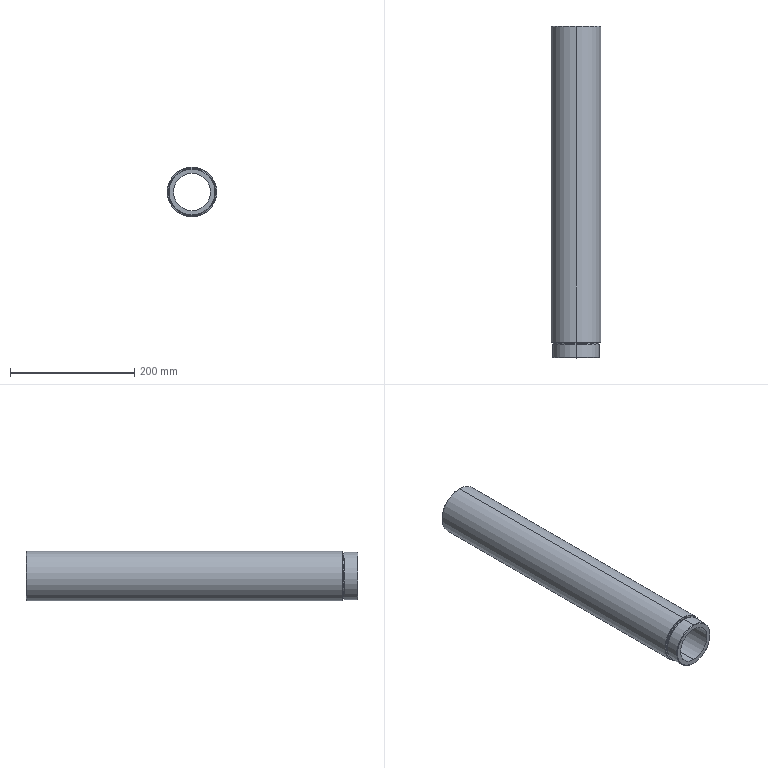Part | SolidWorks | features ICE 8, Chamfer 7, HoleWzd 2, Extrusion 1, Fillet 1 | 1 solid | 33 faces | box 80 x 534.5 x 80 mm | volume 1149532 mm3 | cone 12 | cylinder 12 | plane 5 | torus 4 | commonest cylinder face diameters 60 x2 61 x2 70 x2 73.5 x2 76 x2 80 x2
STEP:
#1=CARTESIAN_POINT('',(0.,529.5,-30.5));
#2=VERTEX_POINT('',#1);
#3=CARTESIAN_POINT('',(0.,529.5,30.5));
#4=VERTEX_POINT('',#3);
#5=CARTESIAN_POINT('',(0.,529.5,0.));
#6=DIRECTION('',(0.,1.,0.));
#7=DIRECTION('',(0.,0.,1.));
#8=AXIS2_PLACEMENT_3D('',#5,#6,#7);
#9=CIRCLE('',#8,30.5);
#10=EDGE_CURVE('',#2,#4,#9,.T.);
#11=ORIENTED_EDGE('',*,*,#10,.F.);
#12=CARTESIAN_POINT('',(0.,530.5,-31.5));
#13=VERTEX_POINT('',#12);
#14=CARTESIAN_POINT('',(0.,529.5,-30.5));
#15=DIRECTION('',(0.,0.7071,-0.7071));
#16=VECTOR('',#15,1000.);
#17=LINE('',#14,#16);
#18=EDGE_CURVE('',#2,#13,#17,.T.);
#19=ORIENTED_EDGE('',*,*,#18,.T.);
#20=CARTESIAN_POINT('',(0.,530.5,31.5));
#21=VERTEX_POINT('',#20);
#22=CARTESIAN_POINT('',(0.,530.5,0.));
#23=DIRECTION('',(0.,-1.,0.));
#24=DIRECTION('',(0.,0.,1.));
#25=AXIS2_PLACEMENT_3D('',#22,#23,#24);
#26=CIRCLE('',#25,31.5);
#27=EDGE_CURVE('',#21,#13,#26,.T.);
#28=ORIENTED_EDGE('',*,*,#27,.F.);
#29=CARTESIAN_POINT('',(0.,529.5,30.5));
#30=DIRECTION('',(0.,0.7071,0.7071));
#31=VECTOR('',#30,1000.);
#32=LINE('',#29,#31);
#33=EDGE_CURVE('',#4,#21,#32,.T.);
#34=ORIENTED_EDGE('',*,*,#33,.F.);
#35=EDGE_LOOP('',(#11,#19,#28,#34));
#36=FACE_OUTER_BOUND('',#35,.T.);
#37=CARTESIAN_POINT('',(0.,529.5,0.));
#38=DIRECTION('',(0.,1.,0.));
#39=DIRECTION('',(0.,0.,1.));
#40=AXIS2_PLACEMENT_3D('',#37,#38,#39);
#41=CONICAL_SURFACE('',#40,30.5,0.7854);
#42=ADVANCED_FACE('',(#36),#41,.F.);
#43=CARTESIAN_POINT('',(0.,475.5,-30.5));
#44=VERTEX_POINT('',#43);
#45=CARTESIAN_POINT('',(0.,475.5,30.5));
#46=VERTEX_POINT('',#45);
#47=CARTESIAN_POINT('',(0.,475.5,0.));
#48=DIRECTION('',(0.,1.,0.));
#49=DIRECTION('',(0.,0.,1.));
#50=AXIS2_PLACEMENT_3D('',#47,#48,#49);
#51=CIRCLE('',#50,30.5);
#52=EDGE_CURVE('',#44,#46,#51,.T.);
#53=ORIENTED_EDGE('',*,*,#52,.F.);
#54=CARTESIAN_POINT('',(0.,530.5,-30.5));
#55=DIRECTION('',(0.,1.,0.));
#56=VECTOR('',#55,1000.);
#57=LINE('',#54,#56);
#58=EDGE_CURVE('',#44,#2,#57,.T.);
#59=ORIENTED_EDGE('',*,*,#58,.T.);
#60=ORIENTED_EDGE('',*,*,#10,.T.);
#61=CARTESIAN_POINT('',(0.,530.5,30.5));
#62=DIRECTION('',(0.,1.,0.));
#63=VECTOR('',#62,1000.);
#64=LINE('',#61,#63);
#65=EDGE_CURVE('',#46,#4,#64,.T.);
#66=ORIENTED_EDGE('',*,*,#65,.F.);
#67=EDGE_LOOP('',(#53,#59,#60,#66));
#68=FACE_OUTER_BOUND('',#67,.T.);
#69=CARTESIAN_POINT('',(0.,530.5,0.));
#70=DIRECTION('',(0.,1.,0.));
#71=DIRECTION('',(0.,0.,1.));
#72=AXIS2_PLACEMENT_3D('',#69,#70,#71);
#73=CYLINDRICAL_SURFACE('',#72,30.5);
#74=ADVANCED_FACE('',(#68),#73,.F.);
#75=CARTESIAN_POINT('',(0.,475.2,30.));
#76=VERTEX_POINT('',#75);
#77=CARTESIAN_POINT('',(0.,475.2,-30.));
#78=VERTEX_POINT('',#77);
#79=CARTESIAN_POINT('',(0.,475.2,0.));
#80=DIRECTION('',(0.,-1.,0.));
#81=DIRECTION('',(0.,0.,1.));
#82=AXIS2_PLACEMENT_3D('',#79,#80,#81);
#83=CIRCLE('',#82,30.);
#84=EDGE_CURVE('',#76,#78,#83,.T.);
#85=ORIENTED_EDGE('',*,*,#84,.T.);
#86=CARTESIAN_POINT('',(0.,475.5,-30.5));
#87=DIRECTION('',(0.,0.515,-0.8572));
#88=VECTOR('',#87,1000.);
#89=LINE('',#86,#88);
#90=EDGE_CURVE('',#78,#44,#89,.T.);
#91=ORIENTED_EDGE('',*,*,#90,.T.);
#92=ORIENTED_EDGE('',*,*,#52,.T.);
#93=CARTESIAN_POINT('',(0.,475.5,30.5));
#94=DIRECTION('',(0.,0.515,0.8572));
#95=VECTOR('',#94,1000.);
#96=LINE('',#93,#95);
#97=EDGE_CURVE('',#76,#46,#96,.T.);
#98=ORIENTED_EDGE('',*,*,#97,.F.);
#99=EDGE_LOOP('',(#85,#91,#92,#98));
#100=FACE_OUTER_BOUND('',#99,.T.);
#101=CARTESIAN_POINT('',(0.,475.5,0.));
#102=DIRECTION('',(0.,1.,0.));
#103=DIRECTION('',(0.,0.,1.));
#104=AXIS2_PLACEMENT_3D('',#101,#102,#103);
#105=CONICAL_SURFACE('',#104,30.5,1.03);
#106=ADVANCED_FACE('',(#100),#105,.F.);
#107=CARTESIAN_POINT('',(0.,27.5,36.75));
#108=VERTEX_POINT('',#107);
#109=CARTESIAN_POINT('',(0.,27.5,-36.75));
#110=VERTEX_POINT('',#109);
#111=CARTESIAN_POINT('',(0.,27.5,0.));
#112=DIRECTION('',(0.,-1.,0.));
#113=DIRECTION('',(0.,0.,-1.));
#114=AXIS2_PLACEMENT_3D('',#111,#112,#113);
#115=CIRCLE('',#114,36.75);
#116=EDGE_CURVE('',#108,#110,#115,.T.);
#117=ORIENTED_EDGE('',*,*,#116,.F.);
#118=CARTESIAN_POINT('',(0.,28.,37.25));
#119=VERTEX_POINT('',#118);
#120=CARTESIAN_POINT('',(0.,27.5,37.25));
#121=DIRECTION('',(1.,0.,0.));
#122=DIRECTION('',(0.,0.,-1.));
#123=AXIS2_PLACEMENT_3D('',#120,#121,#122);
#124=CIRCLE('',#123,0.5);
#125=EDGE_CURVE('',#108,#119,#124,.T.);
#126=ORIENTED_EDGE('',*,*,#125,.T.);
#127=CARTESIAN_POINT('',(0.,28.,-37.25));
#128=VERTEX_POINT('',#127);
#129=CARTESIAN_POINT('',(0.,28.,0.));
#130=DIRECTION('',(0.,1.,0.));
#131=DIRECTION('',(0.,0.,-1.));
#132=AXIS2_PLACEMENT_3D('',#129,#130,#131);
#133=CIRCLE('',#132,37.25);
#134=EDGE_CURVE('',#128,#119,#133,.T.);
#135=ORIENTED_EDGE('',*,*,#134,.F.);
#136=CARTESIAN_POINT('',(0.,27.5,-37.25));
#137=DIRECTION('',(-1.,0.,0.));
#138=DIRECTION('',(0.,0.,1.));
#139=AXIS2_PLACEMENT_3D('',#136,#137,#138);
#140=CIRCLE('',#139,0.5);
#141=EDGE_CURVE('',#110,#128,#140,.T.);
#142=ORIENTED_EDGE('',*,*,#141,.F.);
#143=EDGE_LOOP('',(#117,#126,#135,#142));
#144=FACE_OUTER_BOUND('',#143,.T.);
#145=CARTESIAN_POINT('',(0.,27.5,0.));
#146=DIRECTION('',(0.,-1.,0.));
#147=DIRECTION('',(0.,0.,-1.));
#148=AXIS2_PLACEMENT_3D('',#145,#146,#147);
#149=TOROIDAL_SURFACE('',#148,37.25,0.5);
#150=ADVANCED_FACE('',(#144),#149,.F.);
#151=CARTESIAN_POINT('',(0.,25.,37.25));
#152=VERTEX_POINT('',#151);
#153=CARTESIAN_POINT('',(0.,25.,-37.25));
#154=VERTEX_POINT('',#153);
#155=CARTESIAN_POINT('',(0.,25.,0.));
#156=DIRECTION('',(0.,-1.,0.));
#157=DIRECTION('',(0.,0.,-1.));
#158=AXIS2_PLACEMENT_3D('',#155,#156,#157);
#159=CIRCLE('',#158,37.25);
#160=EDGE_CURVE('',#152,#154,#159,.T.);
#161=ORIENTED_EDGE('',*,*,#160,.F.);
#162=CARTESIAN_POINT('',(0.,25.5,36.75));
#163=VERTEX_POINT('',#162);
#164=CARTESIAN_POINT('',(0.,25.5,37.25));
#165=DIRECTION('',(1.,0.,0.));
#166=DIRECTION('',(0.,0.,-1.));
#167=AXIS2_PLACEMENT_3D('',#164,#165,#166);
#168=CIRCLE('',#167,0.5);
#169=EDGE_CURVE('',#152,#163,#168,.T.);
#170=ORIENTED_EDGE('',*,*,#169,.T.);
#171=CARTESIAN_POINT('',(0.,25.5,-36.75));
#172=VERTEX_POINT('',#171);
#173=CARTESIAN_POINT('',(0.,25.5,0.));
#174=DIRECTION('',(0.,1.,0.));
#175=DIRECTION('',(0.,0.,-1.));
#176=AXIS2_PLACEMENT_3D('',#173,#174,#175);
#177=CIRCLE('',#176,36.75);
#178=EDGE_CURVE('',#172,#163,#177,.T.);
#179=ORIENTED_EDGE('',*,*,#178,.F.);
#180=CARTESIAN_POINT('',(0.,25.5,-37.25));
#181=DIRECTION('',(-1.,0.,0.));
#182=DIRECTION('',(0.,0.,1.));
#183=AXIS2_PLACEMENT_3D('',#180,#181,#182);
#184=CIRCLE('',#183,0.5);
#185=EDGE_CURVE('',#154,#172,#184,.T.);
#186=ORIENTED_EDGE('',*,*,#185,.F.);
#187=EDGE_LOOP('',(#161,#170,#179,#186));
#188=FACE_OUTER_BOUND('',#187,.T.);
#189=CARTESIAN_POINT('',(0.,25.5,0.));
#190=DIRECTION('',(0.,-1.,0.));
#191=DIRECTION('',(0.,0.,-1.));
#192=AXIS2_PLACEMENT_3D('',#189,#190,#191);
#193=TOROIDAL_SURFACE('',#192,37.25,0.5);
#194=ADVANCED_FACE('',(#188),#193,.F.);
#195=CARTESIAN_POINT('',(0.,28.,-39.5));
#196=VERTEX_POINT('',#195);
#197=CARTESIAN_POINT('',(0.,28.,39.5));
#198=VERTEX_POINT('',#197);
#199=CARTESIAN_POINT('',(0.,28.,0.));
#200=DIRECTION('',(0.,-1.,0.));
#201=DIRECTION('',(0.,0.,-1.));
#202=AXIS2_PLACEMENT_3D('',#199,#200,#201);
#203=CIRCLE('',#202,39.5);
#204=EDGE_CURVE('',#196,#198,#203,.T.);
#205=ORIENTED_EDGE('',*,*,#204,.F.);
#206=CARTESIAN_POINT('',(0.,28.5,-40.));
#207=VERTEX_POINT('',#206);
#208=CARTESIAN_POINT('',(0.,28.,-39.5));
#209=DIRECTION('',(0.,0.7071,-0.7071));
#210=VECTOR('',#209,1000.);
#211=LINE('',#208,#210);
#212=EDGE_CURVE('',#196,#207,#211,.T.);
#213=ORIENTED_EDGE('',*,*,#212,.T.);
#214=CARTESIAN_POINT('',(0.,28.5,40.));
#215=VERTEX_POINT('',#214);
#216=CARTESIAN_POINT('',(0.,28.5,0.));
#217=DIRECTION('',(0.,1.,0.));
#218=DIRECTION('',(0.,0.,-1.));
#219=AXIS2_PLACEMENT_3D('',#216,#217,#218);
#220=CIRCLE('',#219,40.);
#221=EDGE_CURVE('',#215,#207,#220,.T.);
#222=ORIENTED_EDGE('',*,*,#221,.F.);
#223=CARTESIAN_POINT('',(0.,28.,39.5));
#224=DIRECTION('',(0.,0.7071,0.7071));
#225=VECTOR('',#224,1000.);
#226=LINE('',#223,#225);
#227=EDGE_CURVE('',#198,#215,#226,.T.);
#228=ORIENTED_EDGE('',*,*,#227,.F.);
#229=EDGE_LOOP('',(#205,#213,#222,#228));
#230=FACE_OUTER_BOUND('',#229,.T.);
#231=CARTESIAN_POINT('',(0.,28.,0.));
#232=DIRECTION('',(0.,1.,0.));
#233=DIRECTION('',(0.,0.,1.));
#234=AXIS2_PLACEMENT_3D('',#231,#232,#233);
#235=CONICAL_SURFACE('',#234,39.5,0.7854);
#236=ADVANCED_FACE('',(#230),#235,.T.);
#237=CARTESIAN_POINT('',(0.,3.,-37.));
#238=VERTEX_POINT('',#237);
#239=CARTESIAN_POINT('',(0.,3.,37.));
#240=VERTEX_POINT('',#239);
#241=CARTESIAN_POINT('',(0.,3.,0.));
#242=DIRECTION('',(0.,-1.,0.));
#243=DIRECTION('',(0.,0.,-1.));
#244=AXIS2_PLACEMENT_3D('',#241,#242,#243);
#245=CIRCLE('',#244,37.);
#246=EDGE_CURVE('',#238,#240,#245,.T.);
#247=ORIENTED_EDGE('',*,*,#246,.F.);
#248=CARTESIAN_POINT('',(0.,4.,-38.));
#249=VERTEX_POINT('',#248);
#250=CARTESIAN_POINT('',(0.,4.,-38.));
#251=DIRECTION('',(0.,0.7071,-0.7071));
#252=VECTOR('',#251,1000.);
#253=LINE('',#250,#252);
#254=EDGE_CURVE('',#238,#249,#253,.T.);
#255=ORIENTED_EDGE('',*,*,#254,.T.);
#256=CARTESIAN_POINT('',(0.,4.,38.));
#257=VERTEX_POINT('',#256);
#258=CARTESIAN_POINT('',(0.,4.,0.));
#259=DIRECTION('',(0.,1.,0.));
#260=DIRECTION('',(0.,0.,-1.));
#261=AXIS2_PLACEMENT_3D('',#258,#259,#260);
#262=CIRCLE('',#261,38.);
#263=EDGE_CURVE('',#257,#249,#262,.T.);
#264=ORIENTED_EDGE('',*,*,#263,.F.);
#265=CARTESIAN_POINT('',(0.,4.,38.));
#266=DIRECTION('',(0.,0.7071,0.7071));
#267=VECTOR('',#266,1000.);
#268=LINE('',#265,#267);
#269=EDGE_CURVE('',#240,#257,#268,.T.);
#270=ORIENTED_EDGE('',*,*,#269,.F.);
#271=EDGE_LOOP('',(#247,#255,#264,#270));
#272=FACE_OUTER_BOUND('',#271,.T.);
#273=CARTESIAN_POINT('',(0.,4.,0.));
#274=DIRECTION('',(0.,1.,0.));
#275=DIRECTION('',(0.,0.,1.));
#276=AXIS2_PLACEMENT_3D('',#273,#274,#275);
#277=CONICAL_SURFACE('',#276,38.,0.7854);
#278=ADVANCED_FACE('',(#272),#277,.T.);
#279=CARTESIAN_POINT('',(0.,537.,-35.));
#280=VERTEX_POINT('',#279);
#281=CARTESIAN_POINT('',(0.,537.,35.));
#282=VERTEX_POINT('',#281);
#283=CARTESIAN_POINT('',(0.,537.,0.));
#284=DIRECTION('',(0.,1.,0.));
#285=DIRECTION('',(0.,0.,1.));
#286=AXIS2_PLACEMENT_3D('',#283,#284,#285);
#287=CIRCLE('',#286,35.);
#288=EDGE_CURVE('',#280,#282,#287,.T.);
#289=ORIENTED_EDGE('',*,*,#288,.F.);
#290=CARTESIAN_POINT('',(0.,537.5,-35.5));
#291=VERTEX_POINT('',#290);
#292=CARTESIAN_POINT('',(0.,537.,-35.));
#293=DIRECTION('',(0.,0.7071,-0.7071));
#294=VECTOR('',#293,1000.);
#295=LINE('',#292,#294);
#296=EDGE_CURVE('',#280,#291,#295,.T.);
#297=ORIENTED_EDGE('',*,*,#296,.T.);
#298=CARTESIAN_POINT('',(0.,537.5,35.5));
#299=VERTEX_POINT('',#298);
#300=CARTESIAN_POINT('',(0.,537.5,0.));
#301=DIRECTION('',(0.,-1.,0.));
#302=DIRECTION('',(0.,0.,1.));
#303=AXIS2_PLACEMENT_3D('',#300,#301,#302);
#304=CIRCLE('',#303,35.5);
#305=EDGE_CURVE('',#299,#291,#304,.T.);
#306=ORIENTED_EDGE('',*,*,#305,.F.);
#307=CARTESIAN_POINT('',(0.,537.,35.));
#308=DIRECTION('',(0.,0.7071,0.7071));
#309=VECTOR('',#308,1000.);
#310=LINE('',#307,#309);
#311=EDGE_CURVE('',#282,#299,#310,.T.);
#312=ORIENTED_EDGE('',*,*,#311,.F.);
#313=EDGE_LOOP('',(#289,#297,#306,#312));
#314=FACE_OUTER_BOUND('',#313,.T.);
#315=CARTESIAN_POINT('',(0.,537.,0.));
#316=DIRECTION('',(0.,1.,0.));
#317=DIRECTION('',(0.,0.,1.));
#318=AXIS2_PLACEMENT_3D('',#315,#316,#317);
#319=CONICAL_SURFACE('',#318,35.,0.7854);
#320=ADVANCED_FACE('',(#314),#319,.F.);
#321=CARTESIAN_POINT('',(0.,530.5,-35.));
#322=VERTEX_POINT('',#321);
#323=CARTESIAN_POINT('',(0.,530.5,35.));
#324=VERTEX_POINT('',#323);
#325=CARTESIAN_POINT('',(0.,530.5,0.));
#326=DIRECTION('',(0.,1.,0.));
#327=DIRECTION('',(0.,0.,1.));
#328=AXIS2_PLACEMENT_3D('',#325,#326,#327);
#329=CIRCLE('',#328,35.);
#330=EDGE_CURVE('',#322,#324,#329,.T.);
#331=ORIENTED_EDGE('',*,*,#330,.F.);
#332=CARTESIAN_POINT('',(0.,530.5,-35.));
#333=DIRECTION('',(0.,1.,0.));
#334=VECTOR('',#333,1000.);
#335=LINE('',#332,#334);
#336=EDGE_CURVE('',#322,#280,#335,.T.);
#337=ORIENTED_EDGE('',*,*,#336,.T.);
#338=ORIENTED_EDGE('',*,*,#288,.T.);
#339=CARTESIAN_POINT('',(0.,530.5,35.));
#340=DIRECTION('',(0.,1.,0.));
#341=VECTOR('',#340,1000.);
#342=LINE('',#339,#341);
#343=EDGE_CURVE('',#324,#282,#342,.T.);
#344=ORIENTED_EDGE('',*,*,#343,.F.);
#345=EDGE_LOOP('',(#331,#337,#338,#344));
#346=FACE_OUTER_BOUND('',#345,.T.);
#347=CARTESIAN_POINT('',(0.,530.5,0.));
#348=DIRECTION('',(0.,1.,0.));
#349=DIRECTION('',(0.,0.,1.));
#350=AXIS2_PLACEMENT_3D('',#347,#348,#349);
#351=CYLINDRICAL_SURFACE('',#350,35.);
#352=ADVANCED_FACE('',(#346),#351,.F.);
#353=CARTESIAN_POINT('',(0.,537.5,39.));
#354=VERTEX_POINT('',#353);
#355=CARTESIAN_POINT('',(0.,537.5,-39.));
#356=VERTEX_POINT('',#355);
#357=CARTESIAN_POINT('',(0.,537.5,0.));
#358=DIRECTION('',(0.,1.,0.));
#359=DIRECTION('',(0.,0.,1.));
#360=AXIS2_PLACEMENT_3D('',#357,#358,#359);
#361=CIRCLE('',#360,39.);
#362=EDGE_CURVE('',#354,#356,#361,.T.);
#363=ORIENTED_EDGE('',*,*,#362,.F.);
#364=CARTESIAN_POINT('',(0.,536.5,40.));
#365=VERTEX_POINT('',#364);
#366=CARTESIAN_POINT('',(0.,537.5,39.));
#367=DIRECTION('',(0.,-0.7071,0.7071));
#368=VECTOR('',#367,1000.);
#369=LINE('',#366,#368);
#370=EDGE_CURVE('',#354,#365,#369,.T.);
#371=ORIENTED_EDGE('',*,*,#370,.T.);
#372=CARTESIAN_POINT('',(0.,536.5,-40.));
#373=VERTEX_POINT('',#372);
#374=CARTESIAN_POINT('',(0.,536.5,0.));
#375=DIRECTION('',(0.,-1.,0.));
#376=DIRECTION('',(0.,0.,1.));
#377=AXIS2_PLACEMENT_3D('',#374,#375,#376);
#378=CIRCLE('',#377,40.);
#379=EDGE_CURVE('',#373,#365,#378,.T.);
#380=ORIENTED_EDGE('',*,*,#379,.F.);
#381=CARTESIAN_POINT('',(0.,537.5,-39.));
#382=DIRECTION('',(0.,-0.7071,-0.7071));
#383=VECTOR('',#382,1000.);
#384=LINE('',#381,#383);
#385=EDGE_CURVE('',#356,#373,#384,.T.);
#386=ORIENTED_EDGE('',*,*,#385,.F.);
#387=EDGE_LOOP('',(#363,#371,#380,#386));
#388=FACE_OUTER_BOUND('',#387,.T.);
#389=CARTESIAN_POINT('',(0.,537.5,0.));
#390=DIRECTION('',(0.,-1.,0.));
#391=DIRECTION('',(0.,0.,-1.));
#392=AXIS2_PLACEMENT_3D('',#389,#390,#391);
#393=CONICAL_SURFACE('',#392,39.,0.7854);
#394=ADVANCED_FACE('',(#388),#393,.T.);
#395=CARTESIAN_POINT('',(0.,27.5,0.));
#396=DIRECTION('',(0.,-1.,0.));
#397=DIRECTION('',(0.,0.,-1.));
#398=AXIS2_PLACEMENT_3D('',#395,#396,#397);
#399=CIRCLE('',#398,36.75);
#400=EDGE_CURVE('',#110,#108,#399,.T.);
#401=ORIENTED_EDGE('',*,*,#400,.T.);
#402=CARTESIAN_POINT('',(0.,28.,36.75));
#403=DIRECTION('',(0.,-1.,0.));
#404=VECTOR('',#403,1000.);
#405=LINE('',#402,#404);
#406=EDGE_CURVE('',#108,#163,#405,.T.);
#407=ORIENTED_EDGE('',*,*,#406,.T.);
#408=CARTESIAN_POINT('',(0.,25.5,0.));
#409=DIRECTION('',(0.,1.,0.));
#410=DIRECTION('',(0.,0.,-1.));
#411=AXIS2_PLACEMENT_3D('',#408,#409,#410);
#412=CIRCLE('',#411,36.75);
#413=EDGE_CURVE('',#163,#172,#412,.T.);
#414=ORIENTED_EDGE('',*,*,#413,.T.);
#415=CARTESIAN_POINT('',(0.,28.,-36.75));
#416=DIRECTION('',(0.,-1.,0.));
#417=VECTOR('',#416,1000.);
#418=LINE('',#415,#417);
#419=EDGE_CURVE('',#110,#172,#418,.T.);
#420=ORIENTED_EDGE('',*,*,#419,.F.);
#421=EDGE_LOOP('',(#401,#407,#414,#420));
#422=FACE_OUTER_BOUND('',#421,.T.);
#423=CARTESIAN_POINT('',(0.,28.,0.));
#424=DIRECTION('',(0.,-1.,0.));
#425=DIRECTION('',(0.,0.,-1.));
#426=AXIS2_PLACEMENT_3D('',#423,#424,#425);
#427=CYLINDRICAL_SURFACE('',#426,36.75);
#428=ADVANCED_FACE('',(#422),#427,.T.);
#429=ORIENTED_EDGE('',*,*,#379,.T.);
#430=CARTESIAN_POINT('',(0.,537.5,40.));
#431=DIRECTION('',(0.,-1.,0.));
#432=VECTOR('',#431,1000.);
#433=LINE('',#430,#432);
#434=EDGE_CURVE('',#365,#215,#433,.T.);
#435=ORIENTED_EDGE('',*,*,#434,.T.);
#436=ORIENTED_EDGE('',*,*,#221,.T.);
#437=CARTESIAN_POINT('',(0.,537.5,-40.));
#438=DIRECTION('',(0.,-1.,0.));
#439=VECTOR('',#438,1000.);
#440=LINE('',#437,#439);
#441=EDGE_CURVE('',#373,#207,#440,.T.);
#442=ORIENTED_EDGE('',*,*,#441,.F.);
#443=EDGE_LOOP('',(#429,#435,#436,#442));
#444=FACE_OUTER_BOUND('',#443,.T.);
#445=CARTESIAN_POINT('',(0.,537.5,0.));
#446=DIRECTION('',(0.,-1.,0.));
#447=DIRECTION('',(0.,0.,-1.));
#448=AXIS2_PLACEMENT_3D('',#445,#446,#447);
#449=CYLINDRICAL_SURFACE('',#448,40.);
#450=ADVANCED_FACE('',(#444),#449,.T.);
#451=CARTESIAN_POINT('',(0.,25.,-38.));
#452=VERTEX_POINT('',#451);
#453=CARTESIAN_POINT('',(0.,25.,38.));
#454=VERTEX_POINT('',#453);
#455=CARTESIAN_POINT('',(0.,25.,0.));
#456=DIRECTION('',(0.,-1.,0.));
#457=DIRECTION('',(0.,0.,-1.));
#458=AXIS2_PLACEMENT_3D('',#455,#456,#457);
#459=CIRCLE('',#458,38.);
#460=EDGE_CURVE('',#452,#454,#459,.T.);
#461=ORIENTED_EDGE('',*,*,#460,.T.);
#462=CARTESIAN_POINT('',(0.,25.,38.));
#463=DIRECTION('',(0.,-1.,0.));
#464=VECTOR('',#463,1000.);
#465=LINE('',#462,#464);
#466=EDGE_CURVE('',#454,#257,#465,.T.);
#467=ORIENTED_EDGE('',*,*,#466,.T.);
#468=ORIENTED_EDGE('',*,*,#263,.T.);
#469=CARTESIAN_POINT('',(0.,25.,-38.));
#470=DIRECTION('',(0.,-1.,0.));
#471=VECTOR('',#470,1000.);
#472=LINE('',#469,#471);
#473=EDGE_CURVE('',#452,#249,#472,.T.);
#474=ORIENTED_EDGE('',*,*,#473,.F.);
#475=EDGE_LOOP('',(#461,#467,#468,#474));
#476=FACE_OUTER_BOUND('',#475,.T.);
#477=CARTESIAN_POINT('',(0.,25.,0.));
#478=DIRECTION('',(0.,-1.,0.));
#479=DIRECTION('',(0.,0.,-1.));
#480=AXIS2_PLACEMENT_3D('',#477,#478,#479);
#481=CYLINDRICAL_SURFACE('',#480,38.);
#482=ADVANCED_FACE('',(#476),#481,.T.);
#483=ORIENTED_EDGE('',*,*,#84,.F.);
#484=CARTESIAN_POINT('',(0.,3.,30.));
#485=VERTEX_POINT('',#484);
#486=CARTESIAN_POINT('',(0.,537.5,30.));
#487=DIRECTION('',(0.,-1.,0.));
#488=VECTOR('',#487,1000.);
#489=LINE('',#486,#488);
#490=EDGE_CURVE('',#76,#485,#489,.T.);
#491=ORIENTED_EDGE('',*,*,#490,.T.);
#492=CARTESIAN_POINT('',(0.,3.,-30.));
#493=VERTEX_POINT('',#492);
#494=CARTESIAN_POINT('',(0.,3.,0.));
#495=DIRECTION('',(0.,-1.,0.));
#496=DIRECTION('',(0.,0.,-1.));
#497=AXIS2_PLACEMENT_3D('',#494,#495,#496);
#498=CIRCLE('',#497,30.);
#499=EDGE_CURVE('',#485,#493,#498,.T.);
#500=ORIENTED_EDGE('',*,*,#499,.T.);
#501=CARTESIAN_POINT('',(0.,537.5,-30.));
#502=DIRECTION('',(0.,-1.,0.));
#503=VECTOR('',#502,1000.);
#504=LINE('',#501,#503);
#505=EDGE_CURVE('',#78,#493,#504,.T.);
#506=ORIENTED_EDGE('',*,*,#505,.F.);
#507=EDGE_LOOP('',(#483,#491,#500,#506));
#508=FACE_OUTER_BOUND('',#507,.T.);
#509=CARTESIAN_POINT('',(0.,537.5,0.));
#510=DIRECTION('',(0.,-1.,0.));
#511=DIRECTION('',(0.,0.,-1.));
#512=AXIS2_PLACEMENT_3D('',#509,#510,#511);
#513=CYLINDRICAL_SURFACE('',#512,30.);
#514=ADVANCED_FACE('',(#508),#513,.F.);
#515=ORIENTED_EDGE('',*,*,#490,.F.);
#516=CARTESIAN_POINT('',(0.,475.2,0.));
#517=DIRECTION('',(0.,-1.,0.));
#518=DIRECTION('',(0.,0.,1.));
#519=AXIS2_PLACEMENT_3D('',#516,#517,#518);
#520=CIRCLE('',#519,30.);
#521=EDGE_CURVE('',#78,#76,#520,.T.);
#522=ORIENTED_EDGE('',*,*,#521,.F.);
#523=ORIENTED_EDGE('',*,*,#505,.T.);
#524=CARTESIAN_POINT('',(0.,3.,0.));
#525=DIRECTION('',(0.,-1.,0.));
#526=DIRECTION('',(0.,0.,-1.));
#527=AXIS2_PLACEMENT_3D('',#524,#525,#526);
#528=CIRCLE('',#527,30.);
#529=EDGE_CURVE('',#493,#485,#528,.T.);
#530=ORIENTED_EDGE('',*,*,#529,.T.);
#531=EDGE_LOOP('',(#515,#522,#523,#530));
#532=FACE_OUTER_BOUND('',#531,.T.);
#533=CARTESIAN_POINT('',(0.,537.5,0.));
#534=DIRECTION('',(0.,-1.,0.));
#535=DIRECTION('',(0.,0.,-1.));
#536=AXIS2_PLACEMENT_3D('',#533,#534,#535);
#537=CYLINDRICAL_SURFACE('',#536,30.);
#538=ADVANCED_FACE('',(#532),#537,.F.);
#539=ORIENTED_EDGE('',*,*,#466,.F.);
#540=CARTESIAN_POINT('',(0.,25.,0.));
#541=DIRECTION('',(0.,-1.,0.));
#542=DIRECTION('',(0.,0.,-1.));
#543=AXIS2_PLACEMENT_3D('',#540,#541,#542);
#544=CIRCLE('',#543,38.);
#545=EDGE_CURVE('',#454,#452,#544,.T.);
#546=ORIENTED_EDGE('',*,*,#545,.T.);
#547=ORIENTED_EDGE('',*,*,#473,.T.);
#548=CARTESIAN_POINT('',(0.,4.,0.));
#549=DIRECTION('',(0.,1.,0.));
#550=DIRECTION('',(0.,0.,-1.));
#551=AXIS2_PLACEMENT_3D('',#548,#549,#550);
#552=CIRCLE('',#551,38.);
#553=EDGE_CURVE('',#249,#257,#552,.T.);
#554=ORIENTED_EDGE('',*,*,#553,.T.);
#555=EDGE_LOOP('',(#539,#546,#547,#554));
#556=FACE_OUTER_BOUND('',#555,.T.);
#557=CARTESIAN_POINT('',(0.,25.,0.));
#558=DIRECTION('',(0.,-1.,0.));
#559=DIRECTION('',(0.,0.,-1.));
#560=AXIS2_PLACEMENT_3D('',#557,#558,#559);
#561=CYLINDRICAL_SURFACE('',#560,38.);
#562=ADVANCED_FACE('',(#556),#561,.T.);
#563=CARTESIAN_POINT('',(0.,25.,0.));
#564=DIRECTION('',(0.,-1.,0.));
#565=DIRECTION('',(0.,0.,-1.));
#566=AXIS2_PLACEMENT_3D('',#563,#564,#565);
#567=CIRCLE('',#566,37.25);
#568=EDGE_CURVE('',#154,#152,#567,.T.);
#569=ORIENTED_EDGE('',*,*,#568,.T.);
#570=ORIENTED_EDGE('',*,*,#160,.T.);
#571=EDGE_LOOP('',(#569,#570));
#572=FACE_BOUND('',#571,.T.);
#573=ORIENTED_EDGE('',*,*,#460,.F.);
#574=ORIENTED_EDGE('',*,*,#545,.F.);
#575=EDGE_LOOP('',(#573,#574));
#576=FACE_OUTER_BOUND('',#575,.T.);
#577=CARTESIAN_POINT('',(0.,25.,0.));
#578=DIRECTION('',(0.,-1.,0.));
#579=DIRECTION('',(0.,0.,-1.));
#580=AXIS2_PLACEMENT_3D('',#577,#578,#579);
#581=PLANE('',#580);
#582=ADVANCED_FACE('',(#572,#576),#581,.F.);
#583=ORIENTED_EDGE('',*,*,#434,.F.);
#584=CARTESIAN_POINT('',(0.,536.5,0.));
#585=DIRECTION('',(0.,-1.,0.));
#586=DIRECTION('',(0.,0.,1.));
#587=AXIS2_PLACEMENT_3D('',#584,#585,#586);
#588=CIRCLE('',#587,40.);
#589=EDGE_CURVE('',#365,#373,#588,.T.);
#590=ORIENTED_EDGE('',*,*,#589,.T.);
#591=ORIENTED_EDGE('',*,*,#441,.T.);
#592=CARTESIAN_POINT('',(0.,28.5,0.));
#593=DIRECTION('',(0.,1.,0.));
#594=DIRECTION('',(0.,0.,-1.));
#595=AXIS2_PLACEMENT_3D('',#592,#593,#594);
#596=CIRCLE('',#595,40.);
#597=EDGE_CURVE('',#207,#215,#596,.T.);
#598=ORIENTED_EDGE('',*,*,#597,.T.);
#599=EDGE_LOOP('',(#583,#590,#591,#598));
#600=FACE_OUTER_BOUND('',#599,.T.);
#601=CARTESIAN_POINT('',(0.,537.5,0.));
#602=DIRECTION('',(0.,-1.,0.));
#603=DIRECTION('',(0.,0.,-1.));
#604=AXIS2_PLACEMENT_3D('',#601,#602,#603);
#605=CYLINDRICAL_SURFACE('',#604,40.);
#606=ADVANCED_FACE('',(#600),#605,.T.);
#607=ORIENTED_EDGE('',*,*,#305,.T.);
#608=CARTESIAN_POINT('',(0.,537.5,0.));
#609=DIRECTION('',(0.,-1.,0.));
#610=DIRECTION('',(0.,0.,1.));
#611=AXIS2_PLACEMENT_3D('',#608,#609,#610);
#612=CIRCLE('',#611,35.5);
#613=EDGE_CURVE('',#291,#299,#612,.T.);
#614=ORIENTED_EDGE('',*,*,#613,.T.);
#615=EDGE_LOOP('',(#607,#614));
#616=FACE_BOUND('',#615,.T.);
#617=CARTESIAN_POINT('',(0.,537.5,0.));
#618=DIRECTION('',(0.,1.,0.));
#619=DIRECTION('',(0.,0.,1.));
#620=AXIS2_PLACEMENT_3D('',#617,#618,#619);
#621=CIRCLE('',#620,39.);
#622=EDGE_CURVE('',#356,#354,#621,.T.);
#623=ORIENTED_EDGE('',*,*,#622,.T.);
#624=ORIENTED_EDGE('',*,*,#362,.T.);
#625=EDGE_LOOP('',(#623,#624));
#626=FACE_OUTER_BOUND('',#625,.T.);
#627=CARTESIAN_POINT('',(0.,537.5,0.));
#628=DIRECTION('',(0.,1.,0.));
#629=DIRECTION('',(0.,0.,1.));
#630=AXIS2_PLACEMENT_3D('',#627,#628,#629);
#631=PLANE('',#630);
#632=ADVANCED_FACE('',(#616,#626),#631,.T.);
#633=ORIENTED_EDGE('',*,*,#134,.T.);
#634=CARTESIAN_POINT('',(0.,28.,0.));
#635=DIRECTION('',(0.,1.,0.));
#636=DIRECTION('',(0.,0.,-1.));
#637=AXIS2_PLACEMENT_3D('',#634,#635,#636);
#638=CIRCLE('',#637,37.25);
#639=EDGE_CURVE('',#119,#128,#638,.T.);
#640=ORIENTED_EDGE('',*,*,#639,.T.);
#641=EDGE_LOOP('',(#633,#640));
#642=FACE_BOUND('',#641,.T.);
#643=CARTESIAN_POINT('',(0.,28.,0.));
#644=DIRECTION('',(0.,-1.,0.));
#645=DIRECTION('',(0.,0.,-1.));
#646=AXIS2_PLACEMENT_3D('',#643,#644,#645);
#647=CIRCLE('',#646,39.5);
#648=EDGE_CURVE('',#198,#196,#647,.T.);
#649=ORIENTED_EDGE('',*,*,#648,.T.);
#650=ORIENTED_EDGE('',*,*,#204,.T.);
#651=EDGE_LOOP('',(#649,#650));
#652=FACE_OUTER_BOUND('',#651,.T.);
#653=CARTESIAN_POINT('',(0.,28.,0.));
#654=DIRECTION('',(0.,-1.,0.));
#655=DIRECTION('',(0.,0.,-1.));
#656=AXIS2_PLACEMENT_3D('',#653,#654,#655);
#657=PLANE('',#656);
#658=ADVANCED_FACE('',(#642,#652),#657,.T.);
#659=ORIENTED_EDGE('',*,*,#406,.F.);
#660=ORIENTED_EDGE('',*,*,#116,.T.);
#661=ORIENTED_EDGE('',*,*,#419,.T.);
#662=ORIENTED_EDGE('',*,*,#178,.T.);
#663=EDGE_LOOP('',(#659,#660,#661,#662));
#664=FACE_OUTER_BOUND('',#663,.T.);
#665=CARTESIAN_POINT('',(0.,28.,0.));
#666=DIRECTION('',(0.,-1.,0.));
#667=DIRECTION('',(0.,0.,-1.));
#668=AXIS2_PLACEMENT_3D('',#665,#666,#667);
#669=CYLINDRICAL_SURFACE('',#668,36.75);
#670=ADVANCED_FACE('',(#664),#669,.T.);
#671=ORIENTED_EDGE('',*,*,#370,.F.);
#672=ORIENTED_EDGE('',*,*,#622,.F.);
#673=ORIENTED_EDGE('',*,*,#385,.T.);
#674=ORIENTED_EDGE('',*,*,#589,.F.);
#675=EDGE_LOOP('',(#671,#672,#673,#674));
#676=FACE_OUTER_BOUND('',#675,.T.);
#677=CARTESIAN_POINT('',(0.,537.5,0.));
#678=DIRECTION('',(0.,-1.,0.));
#679=DIRECTION('',(0.,0.,-1.));
#680=AXIS2_PLACEMENT_3D('',#677,#678,#679);
#681=CONICAL_SURFACE('',#680,39.,0.7854);
#682=ADVANCED_FACE('',(#676),#681,.T.);
#683=ORIENTED_EDGE('',*,*,#336,.F.);
#684=CARTESIAN_POINT('',(0.,530.5,0.));
#685=DIRECTION('',(0.,1.,0.));
#686=DIRECTION('',(0.,0.,1.));
#687=AXIS2_PLACEMENT_3D('',#684,#685,#686);
#688=CIRCLE('',#687,35.);
#689=EDGE_CURVE('',#324,#322,#688,.T.);
#690=ORIENTED_EDGE('',*,*,#689,.F.);
#691=ORIENTED_EDGE('',*,*,#343,.T.);
#692=CARTESIAN_POINT('',(0.,537.,0.));
#693=DIRECTION('',(0.,1.,0.));
#694=DIRECTION('',(0.,0.,1.));
#695=AXIS2_PLACEMENT_3D('',#692,#693,#694);
#696=CIRCLE('',#695,35.);
#697=EDGE_CURVE('',#282,#280,#696,.T.);
#698=ORIENTED_EDGE('',*,*,#697,.T.);
#699=EDGE_LOOP('',(#683,#690,#691,#698));
#700=FACE_OUTER_BOUND('',#699,.T.);
#701=CARTESIAN_POINT('',(0.,530.5,0.));
#702=DIRECTION('',(0.,1.,0.));
#703=DIRECTION('',(0.,0.,1.));
#704=AXIS2_PLACEMENT_3D('',#701,#702,#703);
#705=CYLINDRICAL_SURFACE('',#704,35.);
#706=ADVANCED_FACE('',(#700),#705,.F.);
#707=ORIENTED_EDGE('',*,*,#27,.T.);
#708=CARTESIAN_POINT('',(0.,530.5,0.));
#709=DIRECTION('',(0.,-1.,0.));
#710=DIRECTION('',(0.,0.,1.));
#711=AXIS2_PLACEMENT_3D('',#708,#709,#710);
#712=CIRCLE('',#711,31.5);
#713=EDGE_CURVE('',#13,#21,#712,.T.);
#714=ORIENTED_EDGE('',*,*,#713,.T.);
#715=EDGE_LOOP('',(#707,#714));
#716=FACE_BOUND('',#715,.T.);
#717=ORIENTED_EDGE('',*,*,#689,.T.);
#718=ORIENTED_EDGE('',*,*,#330,.T.);
#719=EDGE_LOOP('',(#717,#718));
#720=FACE_OUTER_BOUND('',#719,.T.);
#721=CARTESIAN_POINT('',(0.,530.5,0.));
#722=DIRECTION('',(0.,1.,0.));
#723=DIRECTION('',(0.,0.,1.));
#724=AXIS2_PLACEMENT_3D('',#721,#722,#723);
#725=PLANE('',#724);
#726=ADVANCED_FACE('',(#716,#720),#725,.T.);
#727=ORIENTED_EDGE('',*,*,#296,.F.);
#728=ORIENTED_EDGE('',*,*,#697,.F.);
#729=ORIENTED_EDGE('',*,*,#311,.T.);
#730=ORIENTED_EDGE('',*,*,#613,.F.);
#731=EDGE_LOOP('',(#727,#728,#729,#730));
#732=FACE_OUTER_BOUND('',#731,.T.);
#733=CARTESIAN_POINT('',(0.,537.,0.));
#734=DIRECTION('',(0.,1.,0.));
#735=DIRECTION('',(0.,0.,1.));
#736=AXIS2_PLACEMENT_3D('',#733,#734,#735);
#737=CONICAL_SURFACE('',#736,35.,0.7854);
#738=ADVANCED_FACE('',(#732),#737,.F.);
#739=CARTESIAN_POINT('',(0.,3.,0.));
#740=DIRECTION('',(0.,-1.,0.));
#741=DIRECTION('',(0.,0.,-1.));
#742=AXIS2_PLACEMENT_3D('',#739,#740,#741);
#743=CIRCLE('',#742,37.);
#744=EDGE_CURVE('',#240,#238,#743,.T.);
#745=ORIENTED_EDGE('',*,*,#744,.T.);
#746=ORIENTED_EDGE('',*,*,#246,.T.);
#747=EDGE_LOOP('',(#745,#746));
#748=FACE_OUTER_BOUND('',#747,.T.);
#749=ORIENTED_EDGE('',*,*,#529,.F.);
#750=ORIENTED_EDGE('',*,*,#499,.F.);
#751=EDGE_LOOP('',(#749,#750));
#752=FACE_BOUND('',#751,.T.);
#753=CARTESIAN_POINT('',(0.,3.,0.));
#754=DIRECTION('',(0.,-1.,0.));
#755=DIRECTION('',(0.,0.,-1.));
#756=AXIS2_PLACEMENT_3D('',#753,#754,#755);
#757=PLANE('',#756);
#758=ADVANCED_FACE('',(#748,#752),#757,.T.);
#759=ORIENTED_EDGE('',*,*,#254,.F.);
#760=ORIENTED_EDGE('',*,*,#744,.F.);
#761=ORIENTED_EDGE('',*,*,#269,.T.);
#762=ORIENTED_EDGE('',*,*,#553,.F.);
#763=EDGE_LOOP('',(#759,#760,#761,#762));
#764=FACE_OUTER_BOUND('',#763,.T.);
#765=CARTESIAN_POINT('',(0.,4.,0.));
#766=DIRECTION('',(0.,1.,0.));
#767=DIRECTION('',(0.,0.,1.));
#768=AXIS2_PLACEMENT_3D('',#765,#766,#767);
#769=CONICAL_SURFACE('',#768,38.,0.7854);
#770=ADVANCED_FACE('',(#764),#769,.T.);
#771=ORIENTED_EDGE('',*,*,#212,.F.);
#772=ORIENTED_EDGE('',*,*,#648,.F.);
#773=ORIENTED_EDGE('',*,*,#227,.T.);
#774=ORIENTED_EDGE('',*,*,#597,.F.);
#775=EDGE_LOOP('',(#771,#772,#773,#774));
#776=FACE_OUTER_BOUND('',#775,.T.);
#777=CARTESIAN_POINT('',(0.,28.,0.));
#778=DIRECTION('',(0.,1.,0.));
#779=DIRECTION('',(0.,0.,1.));
#780=AXIS2_PLACEMENT_3D('',#777,#778,#779);
#781=CONICAL_SURFACE('',#780,39.5,0.7854);
#782=ADVANCED_FACE('',(#776),#781,.T.);
#783=ORIENTED_EDGE('',*,*,#169,.F.);
#784=ORIENTED_EDGE('',*,*,#568,.F.);
#785=ORIENTED_EDGE('',*,*,#185,.T.);
#786=ORIENTED_EDGE('',*,*,#413,.F.);
#787=EDGE_LOOP('',(#783,#784,#785,#786));
#788=FACE_OUTER_BOUND('',#787,.T.);
#789=CARTESIAN_POINT('',(0.,25.5,0.));
#790=DIRECTION('',(0.,-1.,0.));
#791=DIRECTION('',(0.,0.,-1.));
#792=AXIS2_PLACEMENT_3D('',#789,#790,#791);
#793=TOROIDAL_SURFACE('',#792,37.25,0.5);
#794=ADVANCED_FACE('',(#788),#793,.F.);
#795=ORIENTED_EDGE('',*,*,#125,.F.);
#796=ORIENTED_EDGE('',*,*,#400,.F.);
#797=ORIENTED_EDGE('',*,*,#141,.T.);
#798=ORIENTED_EDGE('',*,*,#639,.F.);
#799=EDGE_LOOP('',(#795,#796,#797,#798));
#800=FACE_OUTER_BOUND('',#799,.T.);
#801=CARTESIAN_POINT('',(0.,27.5,0.));
#802=DIRECTION('',(0.,-1.,0.));
#803=DIRECTION('',(0.,0.,-1.));
#804=AXIS2_PLACEMENT_3D('',#801,#802,#803);
#805=TOROIDAL_SURFACE('',#804,37.25,0.5);
#806=ADVANCED_FACE('',(#800),#805,.F.);
#807=ORIENTED_EDGE('',*,*,#90,.F.);
#808=ORIENTED_EDGE('',*,*,#521,.T.);
#809=ORIENTED_EDGE('',*,*,#97,.T.);
#810=CARTESIAN_POINT('',(0.,475.5,0.));
#811=DIRECTION('',(0.,1.,0.));
#812=DIRECTION('',(0.,0.,1.));
#813=AXIS2_PLACEMENT_3D('',#810,#811,#812);
#814=CIRCLE('',#813,30.5);
#815=EDGE_CURVE('',#46,#44,#814,.T.);
#816=ORIENTED_EDGE('',*,*,#815,.T.);
#817=EDGE_LOOP('',(#807,#808,#809,#816));
#818=FACE_OUTER_BOUND('',#817,.T.);
#819=CARTESIAN_POINT('',(0.,475.5,0.));
#820=DIRECTION('',(0.,1.,0.));
#821=DIRECTION('',(0.,0.,1.));
#822=AXIS2_PLACEMENT_3D('',#819,#820,#821);
#823=CONICAL_SURFACE('',#822,30.5,1.03);
#824=ADVANCED_FACE('',(#818),#823,.F.);
#825=ORIENTED_EDGE('',*,*,#58,.F.);
#826=ORIENTED_EDGE('',*,*,#815,.F.);
#827=ORIENTED_EDGE('',*,*,#65,.T.);
#828=CARTESIAN_POINT('',(0.,529.5,0.));
#829=DIRECTION('',(0.,1.,0.));
#830=DIRECTION('',(0.,0.,1.));
#831=AXIS2_PLACEMENT_3D('',#828,#829,#830);
#832=CIRCLE('',#831,30.5);
#833=EDGE_CURVE('',#4,#2,#832,.T.);
#834=ORIENTED_EDGE('',*,*,#833,.T.);
#835=EDGE_LOOP('',(#825,#826,#827,#834));
#836=FACE_OUTER_BOUND('',#835,.T.);
#837=CARTESIAN_POINT('',(0.,530.5,0.));
#838=DIRECTION('',(0.,1.,0.));
#839=DIRECTION('',(0.,0.,1.));
#840=AXIS2_PLACEMENT_3D('',#837,#838,#839);
#841=CYLINDRICAL_SURFACE('',#840,30.5);
#842=ADVANCED_FACE('',(#836),#841,.F.);
#843=ORIENTED_EDGE('',*,*,#18,.F.);
#844=ORIENTED_EDGE('',*,*,#833,.F.);
#845=ORIENTED_EDGE('',*,*,#33,.T.);
#846=ORIENTED_EDGE('',*,*,#713,.F.);
#847=EDGE_LOOP('',(#843,#844,#845,#846));
#848=FACE_OUTER_BOUND('',#847,.T.);
#849=CARTESIAN_POINT('',(0.,529.5,0.));
#850=DIRECTION('',(0.,1.,0.));
#851=DIRECTION('',(0.,0.,1.));
#852=AXIS2_PLACEMENT_3D('',#849,#850,#851);
#853=CONICAL_SURFACE('',#852,30.5,0.7854);
#854=ADVANCED_FACE('',(#848),#853,.F.);
#855=CLOSED_SHELL('',(#42,#74,#106,#150,#194,#236,#278,#320,#352,#394,#428,#450,#482,#514,#538,#562,#582,#606,#632,#658,#670,#682,#706,#726,#738,#758,#770,#782,#794,#806,#824,#842,#854));
#856=MANIFOLD_SOLID_BREP('',#855);
#857=CARTESIAN_POINT('',(0.,0.,0.));
#858=DIRECTION('',(0.,0.,1.));
#859=DIRECTION('',(1.,0.,0.));
#860=AXIS2_PLACEMENT_3D('',#857,#858,#859);
#861=(LENGTH_UNIT()NAMED_UNIT(*)SI_UNIT(.MILLI.,.METRE.));
#862=UNCERTAINTY_MEASURE_WITH_UNIT(LENGTH_MEASURE(0.00001),#861,'','');
#863=(NAMED_UNIT(*)PLANE_ANGLE_UNIT()SI_UNIT($,.RADIAN.));
#864=(NAMED_UNIT(*)SI_UNIT($,.STERADIAN.)SOLID_ANGLE_UNIT());
#865=(GEOMETRIC_REPRESENTATION_CONTEXT(3)GLOBAL_UNCERTAINTY_ASSIGNED_CONTEXT((#862))GLOBAL_UNIT_ASSIGNED_CONTEXT((#861,#863,#864))REPRESENTATION_CONTEXT('',''));
#866=ADVANCED_BREP_SHAPE_REPRESENTATION('',(#856,#860),#865);